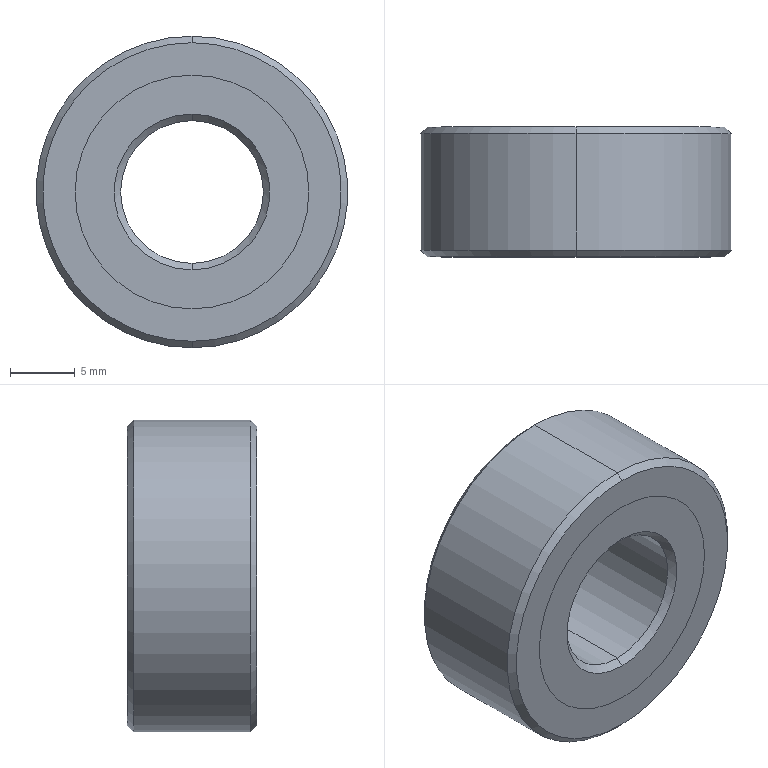Part | SolidWorks | features Chamfer 3, ICE 2, Extrusion 1 | 2 solids | 20 faces | box 24 x 10 x 24 mm | volume 3546 mm3 | cone 8 | cylinder 8 | plane 4 | commonest cylinder face diameters 18 x4 11 x2 24 x2
STEP:
#1=CARTESIAN_POINT('',(0.,0.5,5.5));
#2=VERTEX_POINT('',#1);
#3=CARTESIAN_POINT('',(0.,0.5,-5.5));
#4=VERTEX_POINT('',#3);
#5=CARTESIAN_POINT('',(0.,0.5,0.));
#6=DIRECTION('',(0.,-1.,0.));
#7=DIRECTION('',(0.,0.,1.));
#8=AXIS2_PLACEMENT_3D('',#5,#6,#7);
#9=CIRCLE('',#8,5.5);
#10=EDGE_CURVE('',#2,#4,#9,.T.);
#11=ORIENTED_EDGE('',*,*,#10,.F.);
#12=CARTESIAN_POINT('',(0.,0.,6.));
#13=VERTEX_POINT('',#12);
#14=CARTESIAN_POINT('',(0.,0.,6.));
#15=DIRECTION('',(0.,-0.7071,0.7071));
#16=VECTOR('',#15,1000.);
#17=LINE('',#14,#16);
#18=EDGE_CURVE('',#2,#13,#17,.T.);
#19=ORIENTED_EDGE('',*,*,#18,.T.);
#20=CARTESIAN_POINT('',(0.,0.,-6.));
#21=VERTEX_POINT('',#20);
#22=CARTESIAN_POINT('',(0.,0.,0.));
#23=DIRECTION('',(0.,1.,0.));
#24=DIRECTION('',(0.,0.,1.));
#25=AXIS2_PLACEMENT_3D('',#22,#23,#24);
#26=CIRCLE('',#25,6.);
#27=EDGE_CURVE('',#21,#13,#26,.T.);
#28=ORIENTED_EDGE('',*,*,#27,.F.);
#29=CARTESIAN_POINT('',(0.,0.,-6.));
#30=DIRECTION('',(0.,-0.7071,-0.7071));
#31=VECTOR('',#30,1000.);
#32=LINE('',#29,#31);
#33=EDGE_CURVE('',#4,#21,#32,.T.);
#34=ORIENTED_EDGE('',*,*,#33,.F.);
#35=EDGE_LOOP('',(#11,#19,#28,#34));
#36=FACE_OUTER_BOUND('',#35,.T.);
#37=CARTESIAN_POINT('',(0.,0.,0.));
#38=DIRECTION('',(0.,-1.,0.));
#39=DIRECTION('',(0.,0.,-1.));
#40=AXIS2_PLACEMENT_3D('',#37,#38,#39);
#41=CONICAL_SURFACE('',#40,6.,0.7854);
#42=ADVANCED_FACE('',(#36),#41,.F.);
#43=CARTESIAN_POINT('',(0.,9.5,-5.5));
#44=VERTEX_POINT('',#43);
#45=CARTESIAN_POINT('',(0.,9.5,5.5));
#46=VERTEX_POINT('',#45);
#47=CARTESIAN_POINT('',(0.,9.5,0.));
#48=DIRECTION('',(0.,1.,0.));
#49=DIRECTION('',(0.,0.,1.));
#50=AXIS2_PLACEMENT_3D('',#47,#48,#49);
#51=CIRCLE('',#50,5.5);
#52=EDGE_CURVE('',#44,#46,#51,.T.);
#53=ORIENTED_EDGE('',*,*,#52,.F.);
#54=CARTESIAN_POINT('',(0.,10.,-6.));
#55=VERTEX_POINT('',#54);
#56=CARTESIAN_POINT('',(0.,9.5,-5.5));
#57=DIRECTION('',(0.,0.7071,-0.7071));
#58=VECTOR('',#57,1000.);
#59=LINE('',#56,#58);
#60=EDGE_CURVE('',#44,#55,#59,.T.);
#61=ORIENTED_EDGE('',*,*,#60,.T.);
#62=CARTESIAN_POINT('',(0.,10.,6.));
#63=VERTEX_POINT('',#62);
#64=CARTESIAN_POINT('',(0.,10.,0.));
#65=DIRECTION('',(0.,-1.,0.));
#66=DIRECTION('',(0.,0.,1.));
#67=AXIS2_PLACEMENT_3D('',#64,#65,#66);
#68=CIRCLE('',#67,6.);
#69=EDGE_CURVE('',#63,#55,#68,.T.);
#70=ORIENTED_EDGE('',*,*,#69,.F.);
#71=CARTESIAN_POINT('',(0.,9.5,5.5));
#72=DIRECTION('',(0.,0.7071,0.7071));
#73=VECTOR('',#72,1000.);
#74=LINE('',#71,#73);
#75=EDGE_CURVE('',#46,#63,#74,.T.);
#76=ORIENTED_EDGE('',*,*,#75,.F.);
#77=EDGE_LOOP('',(#53,#61,#70,#76));
#78=FACE_OUTER_BOUND('',#77,.T.);
#79=CARTESIAN_POINT('',(0.,9.5,0.));
#80=DIRECTION('',(0.,1.,0.));
#81=DIRECTION('',(0.,0.,1.));
#82=AXIS2_PLACEMENT_3D('',#79,#80,#81);
#83=CONICAL_SURFACE('',#82,5.5,0.7854);
#84=ADVANCED_FACE('',(#78),#83,.F.);
#85=CARTESIAN_POINT('',(0.,0.,9.));
#86=VERTEX_POINT('',#85);
#87=CARTESIAN_POINT('',(0.,0.,-9.));
#88=VERTEX_POINT('',#87);
#89=CARTESIAN_POINT('',(0.,0.,0.));
#90=DIRECTION('',(0.,1.,0.));
#91=DIRECTION('',(0.,0.,1.));
#92=AXIS2_PLACEMENT_3D('',#89,#90,#91);
#93=CIRCLE('',#92,9.);
#94=EDGE_CURVE('',#86,#88,#93,.T.);
#95=ORIENTED_EDGE('',*,*,#94,.T.);
#96=CARTESIAN_POINT('',(0.,10.,-9.));
#97=VERTEX_POINT('',#96);
#98=CARTESIAN_POINT('',(0.,0.,-9.));
#99=DIRECTION('',(0.,1.,0.));
#100=VECTOR('',#99,1000.);
#101=LINE('',#98,#100);
#102=EDGE_CURVE('',#88,#97,#101,.T.);
#103=ORIENTED_EDGE('',*,*,#102,.T.);
#104=CARTESIAN_POINT('',(0.,10.,9.));
#105=VERTEX_POINT('',#104);
#106=CARTESIAN_POINT('',(0.,10.,0.));
#107=DIRECTION('',(0.,1.,0.));
#108=DIRECTION('',(0.,0.,1.));
#109=AXIS2_PLACEMENT_3D('',#106,#107,#108);
#110=CIRCLE('',#109,9.);
#111=EDGE_CURVE('',#105,#97,#110,.T.);
#112=ORIENTED_EDGE('',*,*,#111,.F.);
#113=CARTESIAN_POINT('',(0.,0.,9.));
#114=DIRECTION('',(0.,1.,0.));
#115=VECTOR('',#114,1000.);
#116=LINE('',#113,#115);
#117=EDGE_CURVE('',#86,#105,#116,.T.);
#118=ORIENTED_EDGE('',*,*,#117,.F.);
#119=EDGE_LOOP('',(#95,#103,#112,#118));
#120=FACE_OUTER_BOUND('',#119,.T.);
#121=CARTESIAN_POINT('',(0.,0.,0.));
#122=DIRECTION('',(0.,1.,0.));
#123=DIRECTION('',(0.,0.,1.));
#124=AXIS2_PLACEMENT_3D('',#121,#122,#123);
#125=CYLINDRICAL_SURFACE('',#124,9.);
#126=ADVANCED_FACE('',(#120),#125,.T.);
#127=ORIENTED_EDGE('',*,*,#52,.T.);
#128=CARTESIAN_POINT('',(0.,10.,5.5));
#129=DIRECTION('',(0.,-1.,0.));
#130=VECTOR('',#129,1000.);
#131=LINE('',#128,#130);
#132=EDGE_CURVE('',#46,#2,#131,.T.);
#133=ORIENTED_EDGE('',*,*,#132,.T.);
#134=ORIENTED_EDGE('',*,*,#10,.T.);
#135=CARTESIAN_POINT('',(0.,10.,-5.5));
#136=DIRECTION('',(0.,-1.,0.));
#137=VECTOR('',#136,1000.);
#138=LINE('',#135,#137);
#139=EDGE_CURVE('',#44,#4,#138,.T.);
#140=ORIENTED_EDGE('',*,*,#139,.F.);
#141=EDGE_LOOP('',(#127,#133,#134,#140));
#142=FACE_OUTER_BOUND('',#141,.T.);
#143=CARTESIAN_POINT('',(0.,10.,0.));
#144=DIRECTION('',(0.,-1.,0.));
#145=DIRECTION('',(0.,0.,-1.));
#146=AXIS2_PLACEMENT_3D('',#143,#144,#145);
#147=CYLINDRICAL_SURFACE('',#146,5.5);
#148=ADVANCED_FACE('',(#142),#147,.F.);
#149=ORIENTED_EDGE('',*,*,#69,.T.);
#150=CARTESIAN_POINT('',(0.,10.,0.));
#151=DIRECTION('',(0.,-1.,0.));
#152=DIRECTION('',(0.,0.,1.));
#153=AXIS2_PLACEMENT_3D('',#150,#151,#152);
#154=CIRCLE('',#153,6.);
#155=EDGE_CURVE('',#55,#63,#154,.T.);
#156=ORIENTED_EDGE('',*,*,#155,.T.);
#157=EDGE_LOOP('',(#149,#156));
#158=FACE_BOUND('',#157,.T.);
#159=ORIENTED_EDGE('',*,*,#111,.T.);
#160=CARTESIAN_POINT('',(0.,10.,0.));
#161=DIRECTION('',(0.,1.,0.));
#162=DIRECTION('',(0.,0.,1.));
#163=AXIS2_PLACEMENT_3D('',#160,#161,#162);
#164=CIRCLE('',#163,9.);
#165=EDGE_CURVE('',#97,#105,#164,.T.);
#166=ORIENTED_EDGE('',*,*,#165,.T.);
#167=EDGE_LOOP('',(#159,#166));
#168=FACE_OUTER_BOUND('',#167,.T.);
#169=CARTESIAN_POINT('',(0.,10.,0.));
#170=DIRECTION('',(0.,1.,0.));
#171=DIRECTION('',(0.,0.,1.));
#172=AXIS2_PLACEMENT_3D('',#169,#170,#171);
#173=PLANE('',#172);
#174=ADVANCED_FACE('',(#158,#168),#173,.T.);
#175=ORIENTED_EDGE('',*,*,#27,.T.);
#176=CARTESIAN_POINT('',(0.,0.,0.));
#177=DIRECTION('',(0.,1.,0.));
#178=DIRECTION('',(0.,0.,1.));
#179=AXIS2_PLACEMENT_3D('',#176,#177,#178);
#180=CIRCLE('',#179,6.);
#181=EDGE_CURVE('',#13,#21,#180,.T.);
#182=ORIENTED_EDGE('',*,*,#181,.T.);
#183=EDGE_LOOP('',(#175,#182));
#184=FACE_BOUND('',#183,.T.);
#185=ORIENTED_EDGE('',*,*,#94,.F.);
#186=CARTESIAN_POINT('',(0.,0.,0.));
#187=DIRECTION('',(0.,1.,0.));
#188=DIRECTION('',(0.,0.,1.));
#189=AXIS2_PLACEMENT_3D('',#186,#187,#188);
#190=CIRCLE('',#189,9.);
#191=EDGE_CURVE('',#88,#86,#190,.T.);
#192=ORIENTED_EDGE('',*,*,#191,.F.);
#193=EDGE_LOOP('',(#185,#192));
#194=FACE_OUTER_BOUND('',#193,.T.);
#195=CARTESIAN_POINT('',(0.,0.,0.));
#196=DIRECTION('',(0.,1.,0.));
#197=DIRECTION('',(0.,0.,1.));
#198=AXIS2_PLACEMENT_3D('',#195,#196,#197);
#199=PLANE('',#198);
#200=ADVANCED_FACE('',(#184,#194),#199,.F.);
#201=ORIENTED_EDGE('',*,*,#132,.F.);
#202=CARTESIAN_POINT('',(0.,9.5,0.));
#203=DIRECTION('',(0.,1.,0.));
#204=DIRECTION('',(0.,0.,1.));
#205=AXIS2_PLACEMENT_3D('',#202,#203,#204);
#206=CIRCLE('',#205,5.5);
#207=EDGE_CURVE('',#46,#44,#206,.T.);
#208=ORIENTED_EDGE('',*,*,#207,.T.);
#209=ORIENTED_EDGE('',*,*,#139,.T.);
#210=CARTESIAN_POINT('',(0.,0.5,0.));
#211=DIRECTION('',(0.,-1.,0.));
#212=DIRECTION('',(0.,0.,1.));
#213=AXIS2_PLACEMENT_3D('',#210,#211,#212);
#214=CIRCLE('',#213,5.5);
#215=EDGE_CURVE('',#4,#2,#214,.T.);
#216=ORIENTED_EDGE('',*,*,#215,.T.);
#217=EDGE_LOOP('',(#201,#208,#209,#216));
#218=FACE_OUTER_BOUND('',#217,.T.);
#219=CARTESIAN_POINT('',(0.,10.,0.));
#220=DIRECTION('',(0.,-1.,0.));
#221=DIRECTION('',(0.,0.,-1.));
#222=AXIS2_PLACEMENT_3D('',#219,#220,#221);
#223=CYLINDRICAL_SURFACE('',#222,5.5);
#224=ADVANCED_FACE('',(#218),#223,.F.);
#225=ORIENTED_EDGE('',*,*,#102,.F.);
#226=ORIENTED_EDGE('',*,*,#191,.T.);
#227=ORIENTED_EDGE('',*,*,#117,.T.);
#228=ORIENTED_EDGE('',*,*,#165,.F.);
#229=EDGE_LOOP('',(#225,#226,#227,#228));
#230=FACE_OUTER_BOUND('',#229,.T.);
#231=CARTESIAN_POINT('',(0.,0.,0.));
#232=DIRECTION('',(0.,1.,0.));
#233=DIRECTION('',(0.,0.,1.));
#234=AXIS2_PLACEMENT_3D('',#231,#232,#233);
#235=CYLINDRICAL_SURFACE('',#234,9.);
#236=ADVANCED_FACE('',(#230),#235,.T.);
#237=ORIENTED_EDGE('',*,*,#60,.F.);
#238=ORIENTED_EDGE('',*,*,#207,.F.);
#239=ORIENTED_EDGE('',*,*,#75,.T.);
#240=ORIENTED_EDGE('',*,*,#155,.F.);
#241=EDGE_LOOP('',(#237,#238,#239,#240));
#242=FACE_OUTER_BOUND('',#241,.T.);
#243=CARTESIAN_POINT('',(0.,9.5,0.));
#244=DIRECTION('',(0.,1.,0.));
#245=DIRECTION('',(0.,0.,1.));
#246=AXIS2_PLACEMENT_3D('',#243,#244,#245);
#247=CONICAL_SURFACE('',#246,5.5,0.7854);
#248=ADVANCED_FACE('',(#242),#247,.F.);
#249=ORIENTED_EDGE('',*,*,#18,.F.);
#250=ORIENTED_EDGE('',*,*,#215,.F.);
#251=ORIENTED_EDGE('',*,*,#33,.T.);
#252=ORIENTED_EDGE('',*,*,#181,.F.);
#253=EDGE_LOOP('',(#249,#250,#251,#252));
#254=FACE_OUTER_BOUND('',#253,.T.);
#255=CARTESIAN_POINT('',(0.,0.,0.));
#256=DIRECTION('',(0.,-1.,0.));
#257=DIRECTION('',(0.,0.,-1.));
#258=AXIS2_PLACEMENT_3D('',#255,#256,#257);
#259=CONICAL_SURFACE('',#258,6.,0.7854);
#260=ADVANCED_FACE('',(#254),#259,.F.);
#261=CLOSED_SHELL('',(#42,#84,#126,#148,#174,#200,#224,#236,#248,#260));
#262=MANIFOLD_SOLID_BREP('',#261);
#263=CARTESIAN_POINT('',(0.,10.,11.5));
#264=VERTEX_POINT('',#263);
#265=CARTESIAN_POINT('',(0.,10.,-11.5));
#266=VERTEX_POINT('',#265);
#267=CARTESIAN_POINT('',(0.,10.,0.));
#268=DIRECTION('',(0.,1.,0.));
#269=DIRECTION('',(0.,0.,1.));
#270=AXIS2_PLACEMENT_3D('',#267,#268,#269);
#271=CIRCLE('',#270,11.5);
#272=EDGE_CURVE('',#264,#266,#271,.T.);
#273=ORIENTED_EDGE('',*,*,#272,.F.);
#274=CARTESIAN_POINT('',(0.,9.5,12.));
#275=VERTEX_POINT('',#274);
#276=CARTESIAN_POINT('',(0.,10.,11.5));
#277=DIRECTION('',(0.,-0.7071,0.7071));
#278=VECTOR('',#277,1000.);
#279=LINE('',#276,#278);
#280=EDGE_CURVE('',#264,#275,#279,.T.);
#281=ORIENTED_EDGE('',*,*,#280,.T.);
#282=CARTESIAN_POINT('',(0.,9.5,-12.));
#283=VERTEX_POINT('',#282);
#284=CARTESIAN_POINT('',(0.,9.5,0.));
#285=DIRECTION('',(0.,-1.,0.));
#286=DIRECTION('',(0.,0.,1.));
#287=AXIS2_PLACEMENT_3D('',#284,#285,#286);
#288=CIRCLE('',#287,12.);
#289=EDGE_CURVE('',#283,#275,#288,.T.);
#290=ORIENTED_EDGE('',*,*,#289,.F.);
#291=CARTESIAN_POINT('',(0.,10.,-11.5));
#292=DIRECTION('',(0.,-0.7071,-0.7071));
#293=VECTOR('',#292,1000.);
#294=LINE('',#291,#293);
#295=EDGE_CURVE('',#266,#283,#294,.T.);
#296=ORIENTED_EDGE('',*,*,#295,.F.);
#297=EDGE_LOOP('',(#273,#281,#290,#296));
#298=FACE_OUTER_BOUND('',#297,.T.);
#299=CARTESIAN_POINT('',(0.,10.,0.));
#300=DIRECTION('',(0.,-1.,0.));
#301=DIRECTION('',(0.,0.,-1.));
#302=AXIS2_PLACEMENT_3D('',#299,#300,#301);
#303=CONICAL_SURFACE('',#302,11.5,0.7854);
#304=ADVANCED_FACE('',(#298),#303,.T.);
#305=CARTESIAN_POINT('',(0.,0.,-11.5));
#306=VERTEX_POINT('',#305);
#307=CARTESIAN_POINT('',(0.,0.,11.5));
#308=VERTEX_POINT('',#307);
#309=CARTESIAN_POINT('',(0.,0.,0.));
#310=DIRECTION('',(0.,-1.,0.));
#311=DIRECTION('',(0.,0.,1.));
#312=AXIS2_PLACEMENT_3D('',#309,#310,#311);
#313=CIRCLE('',#312,11.5);
#314=EDGE_CURVE('',#306,#308,#313,.T.);
#315=ORIENTED_EDGE('',*,*,#314,.F.);
#316=CARTESIAN_POINT('',(0.,0.5,-12.));
#317=VERTEX_POINT('',#316);
#318=CARTESIAN_POINT('',(0.,0.,-11.5));
#319=DIRECTION('',(0.,0.7071,-0.7071));
#320=VECTOR('',#319,1000.);
#321=LINE('',#318,#320);
#322=EDGE_CURVE('',#306,#317,#321,.T.);
#323=ORIENTED_EDGE('',*,*,#322,.T.);
#324=CARTESIAN_POINT('',(0.,0.5,12.));
#325=VERTEX_POINT('',#324);
#326=CARTESIAN_POINT('',(0.,0.5,0.));
#327=DIRECTION('',(0.,1.,0.));
#328=DIRECTION('',(0.,0.,1.));
#329=AXIS2_PLACEMENT_3D('',#326,#327,#328);
#330=CIRCLE('',#329,12.);
#331=EDGE_CURVE('',#325,#317,#330,.T.);
#332=ORIENTED_EDGE('',*,*,#331,.F.);
#333=CARTESIAN_POINT('',(0.,0.,11.5));
#334=DIRECTION('',(0.,0.7071,0.7071));
#335=VECTOR('',#334,1000.);
#336=LINE('',#333,#335);
#337=EDGE_CURVE('',#308,#325,#336,.T.);
#338=ORIENTED_EDGE('',*,*,#337,.F.);
#339=EDGE_LOOP('',(#315,#323,#332,#338));
#340=FACE_OUTER_BOUND('',#339,.T.);
#341=CARTESIAN_POINT('',(0.,0.,0.));
#342=DIRECTION('',(0.,1.,0.));
#343=DIRECTION('',(0.,0.,1.));
#344=AXIS2_PLACEMENT_3D('',#341,#342,#343);
#345=CONICAL_SURFACE('',#344,11.5,0.7854);
#346=ADVANCED_FACE('',(#340),#345,.T.);
#347=CARTESIAN_POINT('',(0.,0.,9.));
#348=VERTEX_POINT('',#347);
#349=CARTESIAN_POINT('',(0.,0.,-9.));
#350=VERTEX_POINT('',#349);
#351=CARTESIAN_POINT('',(0.,0.,0.));
#352=DIRECTION('',(0.,-1.,0.));
#353=DIRECTION('',(0.,0.,1.));
#354=AXIS2_PLACEMENT_3D('',#351,#352,#353);
#355=CIRCLE('',#354,9.);
#356=EDGE_CURVE('',#348,#350,#355,.T.);
#357=ORIENTED_EDGE('',*,*,#356,.T.);
#358=CARTESIAN_POINT('',(0.,10.,-9.));
#359=VERTEX_POINT('',#358);
#360=CARTESIAN_POINT('',(0.,-33.941,-9.));
#361=DIRECTION('',(0.,1.,0.));
#362=VECTOR('',#361,1000.);
#363=LINE('',#360,#362);
#364=EDGE_CURVE('',#350,#359,#363,.T.);
#365=ORIENTED_EDGE('',*,*,#364,.T.);
#366=CARTESIAN_POINT('',(0.,10.,9.));
#367=VERTEX_POINT('',#366);
#368=CARTESIAN_POINT('',(0.,10.,0.));
#369=DIRECTION('',(0.,1.,0.));
#370=DIRECTION('',(0.,0.,1.));
#371=AXIS2_PLACEMENT_3D('',#368,#369,#370);
#372=CIRCLE('',#371,9.);
#373=EDGE_CURVE('',#359,#367,#372,.T.);
#374=ORIENTED_EDGE('',*,*,#373,.T.);
#375=CARTESIAN_POINT('',(0.,-33.941,9.));
#376=DIRECTION('',(0.,1.,0.));
#377=VECTOR('',#376,1000.);
#378=LINE('',#375,#377);
#379=EDGE_CURVE('',#348,#367,#378,.T.);
#380=ORIENTED_EDGE('',*,*,#379,.F.);
#381=EDGE_LOOP('',(#357,#365,#374,#380));
#382=FACE_OUTER_BOUND('',#381,.T.);
#383=CARTESIAN_POINT('',(0.,-33.941,0.));
#384=DIRECTION('',(0.,1.,0.));
#385=DIRECTION('',(0.,0.,1.));
#386=AXIS2_PLACEMENT_3D('',#383,#384,#385);
#387=CYLINDRICAL_SURFACE('',#386,9.);
#388=ADVANCED_FACE('',(#382),#387,.F.);
#389=ORIENTED_EDGE('',*,*,#331,.T.);
#390=CARTESIAN_POINT('',(0.,-33.941,-12.));
#391=DIRECTION('',(0.,1.,0.));
#392=VECTOR('',#391,1000.);
#393=LINE('',#390,#392);
#394=EDGE_CURVE('',#317,#283,#393,.T.);
#395=ORIENTED_EDGE('',*,*,#394,.T.);
#396=ORIENTED_EDGE('',*,*,#289,.T.);
#397=CARTESIAN_POINT('',(0.,-33.941,12.));
#398=DIRECTION('',(0.,1.,0.));
#399=VECTOR('',#398,1000.);
#400=LINE('',#397,#399);
#401=EDGE_CURVE('',#325,#275,#400,.T.);
#402=ORIENTED_EDGE('',*,*,#401,.F.);
#403=EDGE_LOOP('',(#389,#395,#396,#402));
#404=FACE_OUTER_BOUND('',#403,.T.);
#405=CARTESIAN_POINT('',(0.,-33.941,0.));
#406=DIRECTION('',(0.,1.,0.));
#407=DIRECTION('',(0.,0.,1.));
#408=AXIS2_PLACEMENT_3D('',#405,#406,#407);
#409=CYLINDRICAL_SURFACE('',#408,12.);
#410=ADVANCED_FACE('',(#404),#409,.T.);
#411=ORIENTED_EDGE('',*,*,#394,.F.);
#412=CARTESIAN_POINT('',(0.,0.5,0.));
#413=DIRECTION('',(0.,1.,0.));
#414=DIRECTION('',(0.,0.,1.));
#415=AXIS2_PLACEMENT_3D('',#412,#413,#414);
#416=CIRCLE('',#415,12.);
#417=EDGE_CURVE('',#317,#325,#416,.T.);
#418=ORIENTED_EDGE('',*,*,#417,.T.);
#419=ORIENTED_EDGE('',*,*,#401,.T.);
#420=CARTESIAN_POINT('',(0.,9.5,0.));
#421=DIRECTION('',(0.,-1.,0.));
#422=DIRECTION('',(0.,0.,1.));
#423=AXIS2_PLACEMENT_3D('',#420,#421,#422);
#424=CIRCLE('',#423,12.);
#425=EDGE_CURVE('',#275,#283,#424,.T.);
#426=ORIENTED_EDGE('',*,*,#425,.T.);
#427=EDGE_LOOP('',(#411,#418,#419,#426));
#428=FACE_OUTER_BOUND('',#427,.T.);
#429=CARTESIAN_POINT('',(0.,-33.941,0.));
#430=DIRECTION('',(0.,1.,0.));
#431=DIRECTION('',(0.,0.,1.));
#432=AXIS2_PLACEMENT_3D('',#429,#430,#431);
#433=CYLINDRICAL_SURFACE('',#432,12.);
#434=ADVANCED_FACE('',(#428),#433,.T.);
#435=CARTESIAN_POINT('',(0.,10.,0.));
#436=DIRECTION('',(0.,1.,0.));
#437=DIRECTION('',(0.,0.,1.));
#438=AXIS2_PLACEMENT_3D('',#435,#436,#437);
#439=CIRCLE('',#438,11.5);
#440=EDGE_CURVE('',#266,#264,#439,.T.);
#441=ORIENTED_EDGE('',*,*,#440,.T.);
#442=ORIENTED_EDGE('',*,*,#272,.T.);
#443=EDGE_LOOP('',(#441,#442));
#444=FACE_OUTER_BOUND('',#443,.T.);
#445=CARTESIAN_POINT('',(0.,10.,0.));
#446=DIRECTION('',(0.,1.,0.));
#447=DIRECTION('',(0.,0.,1.));
#448=AXIS2_PLACEMENT_3D('',#445,#446,#447);
#449=CIRCLE('',#448,9.);
#450=EDGE_CURVE('',#367,#359,#449,.T.);
#451=ORIENTED_EDGE('',*,*,#450,.F.);
#452=ORIENTED_EDGE('',*,*,#373,.F.);
#453=EDGE_LOOP('',(#451,#452));
#454=FACE_BOUND('',#453,.T.);
#455=CARTESIAN_POINT('',(0.,10.,0.));
#456=DIRECTION('',(0.,1.,0.));
#457=DIRECTION('',(0.,0.,1.));
#458=AXIS2_PLACEMENT_3D('',#455,#456,#457);
#459=PLANE('',#458);
#460=ADVANCED_FACE('',(#444,#454),#459,.T.);
#461=ORIENTED_EDGE('',*,*,#364,.F.);
#462=CARTESIAN_POINT('',(0.,0.,0.));
#463=DIRECTION('',(0.,-1.,0.));
#464=DIRECTION('',(0.,0.,1.));
#465=AXIS2_PLACEMENT_3D('',#462,#463,#464);
#466=CIRCLE('',#465,9.);
#467=EDGE_CURVE('',#350,#348,#466,.T.);
#468=ORIENTED_EDGE('',*,*,#467,.T.);
#469=ORIENTED_EDGE('',*,*,#379,.T.);
#470=ORIENTED_EDGE('',*,*,#450,.T.);
#471=EDGE_LOOP('',(#461,#468,#469,#470));
#472=FACE_OUTER_BOUND('',#471,.T.);
#473=CARTESIAN_POINT('',(0.,-33.941,0.));
#474=DIRECTION('',(0.,1.,0.));
#475=DIRECTION('',(0.,0.,1.));
#476=AXIS2_PLACEMENT_3D('',#473,#474,#475);
#477=CYLINDRICAL_SURFACE('',#476,9.);
#478=ADVANCED_FACE('',(#472),#477,.F.);
#479=CARTESIAN_POINT('',(0.,0.,0.));
#480=DIRECTION('',(0.,-1.,0.));
#481=DIRECTION('',(0.,0.,1.));
#482=AXIS2_PLACEMENT_3D('',#479,#480,#481);
#483=CIRCLE('',#482,11.5);
#484=EDGE_CURVE('',#308,#306,#483,.T.);
#485=ORIENTED_EDGE('',*,*,#484,.T.);
#486=ORIENTED_EDGE('',*,*,#314,.T.);
#487=EDGE_LOOP('',(#485,#486));
#488=FACE_OUTER_BOUND('',#487,.T.);
#489=ORIENTED_EDGE('',*,*,#356,.F.);
#490=ORIENTED_EDGE('',*,*,#467,.F.);
#491=EDGE_LOOP('',(#489,#490));
#492=FACE_BOUND('',#491,.T.);
#493=CARTESIAN_POINT('',(0.,0.,0.));
#494=DIRECTION('',(0.,1.,0.));
#495=DIRECTION('',(0.,0.,1.));
#496=AXIS2_PLACEMENT_3D('',#493,#494,#495);
#497=PLANE('',#496);
#498=ADVANCED_FACE('',(#488,#492),#497,.F.);
#499=ORIENTED_EDGE('',*,*,#322,.F.);
#500=ORIENTED_EDGE('',*,*,#484,.F.);
#501=ORIENTED_EDGE('',*,*,#337,.T.);
#502=ORIENTED_EDGE('',*,*,#417,.F.);
#503=EDGE_LOOP('',(#499,#500,#501,#502));
#504=FACE_OUTER_BOUND('',#503,.T.);
#505=CARTESIAN_POINT('',(0.,0.,0.));
#506=DIRECTION('',(0.,1.,0.));
#507=DIRECTION('',(0.,0.,1.));
#508=AXIS2_PLACEMENT_3D('',#505,#506,#507);
#509=CONICAL_SURFACE('',#508,11.5,0.7854);
#510=ADVANCED_FACE('',(#504),#509,.T.);
#511=ORIENTED_EDGE('',*,*,#280,.F.);
#512=ORIENTED_EDGE('',*,*,#440,.F.);
#513=ORIENTED_EDGE('',*,*,#295,.T.);
#514=ORIENTED_EDGE('',*,*,#425,.F.);
#515=EDGE_LOOP('',(#511,#512,#513,#514));
#516=FACE_OUTER_BOUND('',#515,.T.);
#517=CARTESIAN_POINT('',(0.,10.,0.));
#518=DIRECTION('',(0.,-1.,0.));
#519=DIRECTION('',(0.,0.,-1.));
#520=AXIS2_PLACEMENT_3D('',#517,#518,#519);
#521=CONICAL_SURFACE('',#520,11.5,0.7854);
#522=ADVANCED_FACE('',(#516),#521,.T.);
#523=CLOSED_SHELL('',(#304,#346,#388,#410,#434,#460,#478,#498,#510,#522));
#524=MANIFOLD_SOLID_BREP('',#523);
#525=CARTESIAN_POINT('',(0.,0.,0.));
#526=DIRECTION('',(0.,0.,1.));
#527=DIRECTION('',(1.,0.,0.));
#528=AXIS2_PLACEMENT_3D('',#525,#526,#527);
#529=(LENGTH_UNIT()NAMED_UNIT(*)SI_UNIT(.MILLI.,.METRE.));
#530=UNCERTAINTY_MEASURE_WITH_UNIT(LENGTH_MEASURE(0.00001),#529,'','');
#531=(NAMED_UNIT(*)PLANE_ANGLE_UNIT()SI_UNIT($,.RADIAN.));
#532=(NAMED_UNIT(*)SI_UNIT($,.STERADIAN.)SOLID_ANGLE_UNIT());
#533=(GEOMETRIC_REPRESENTATION_CONTEXT(3)GLOBAL_UNCERTAINTY_ASSIGNED_CONTEXT((#530))GLOBAL_UNIT_ASSIGNED_CONTEXT((#529,#531,#532))REPRESENTATION_CONTEXT('',''));
#534=ADVANCED_BREP_SHAPE_REPRESENTATION('',(#262,#524,#528),#533);